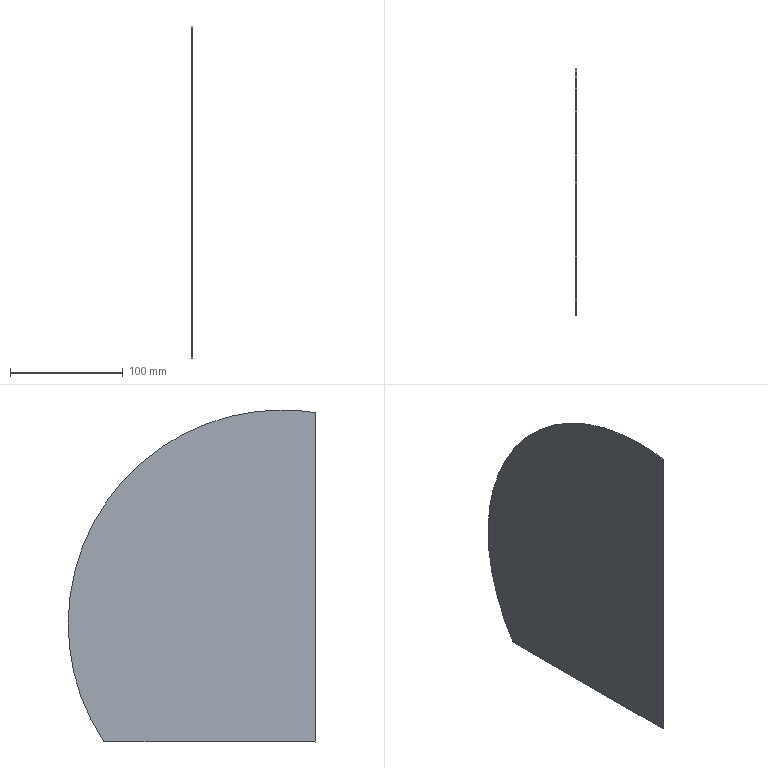Part | STEP file | 09-03 Inner base plate 2 | 1 solid | 6 faces | box 1 x 220 x 295 mm | volume 56061 mm3 | plane 4 | cylinder 2 | commonest cylinder face diameters 380 x2
STEP:
#1=CARTESIAN_POINT('',(0.,0.,0.));
#2=DIRECTION('',(0.,0.,1.));
#3=DIRECTION('',(1.,0.,0.));
#4=AXIS2_PLACEMENT_3D('',#1,#2,#3);
#5=CARTESIAN_POINT('',(1.,30.,295.));
#6=VERTEX_POINT('',#5);
#7=CARTESIAN_POINT('',(1.,0.,292.617));
#8=VERTEX_POINT('',#7);
#9=CARTESIAN_POINT('',(1.,30.,105.));
#10=DIRECTION('',(1.,0.,0.));
#11=DIRECTION('',(0.,0.,1.));
#12=AXIS2_PLACEMENT_3D('',#9,#10,#11);
#13=CIRCLE('',#12,190.);
#14=CARTESIAN_POINT('',(1.,30.,105.));
#15=DIRECTION('',(-1.,0.,0.));
#16=DIRECTION('',(0.,0.,1.));
#17=AXIS2_PLACEMENT_3D('',#14,#15,#16);
#18=CYLINDRICAL_SURFACE('',#17,190.);
#19=CARTESIAN_POINT('',(6.283,0.));
#20=DIRECTION('',(-1.,0.));
#21=VECTOR('',#20,1.);
#22=LINE('',#19,#21);
#23=(GEOMETRIC_REPRESENTATION_CONTEXT(2)PARAMETRIC_REPRESENTATION_CONTEXT()REPRESENTATION_CONTEXT('',''));
#24=DEFINITIONAL_REPRESENTATION('',(#22),#23);
#25=PCURVE('',#18,#24);
#26=CARTESIAN_POINT('',(1.,0.,296.77));
#27=DIRECTION('',(1.,0.,0.));
#28=DIRECTION('',(0.,0.,-1.));
#29=AXIS2_PLACEMENT_3D('',#26,#27,#28);
#30=PLANE('',#29);
#31=CARTESIAN_POINT('',(191.77,30.));
#32=DIRECTION('',(-1.,0.));
#33=AXIS2_PLACEMENT_2D('',#31,#32);
#34=CIRCLE('',#33,190.);
#35=(GEOMETRIC_REPRESENTATION_CONTEXT(2)PARAMETRIC_REPRESENTATION_CONTEXT()REPRESENTATION_CONTEXT('',''));
#36=DEFINITIONAL_REPRESENTATION('',(#34),#35);
#37=PCURVE('',#30,#36);
#38=SURFACE_CURVE('',#13,(#25,#37),.PCURVE_S1.);
#39=EDGE_CURVE('',#6,#8,#38,.T.);
#40=ORIENTED_EDGE('',*,*,#39,.F.);
#41=CARTESIAN_POINT('',(0.,30.,295.));
#42=VERTEX_POINT('',#41);
#43=CARTESIAN_POINT('',(1.,30.,295.));
#44=DIRECTION('',(-1.,0.,0.));
#45=VECTOR('',#44,1.);
#46=LINE('',#43,#45);
#47=CARTESIAN_POINT('',(6.283,0.));
#48=DIRECTION('',(0.,1.));
#49=VECTOR('',#48,1.);
#50=LINE('',#47,#49);
#51=(GEOMETRIC_REPRESENTATION_CONTEXT(2)PARAMETRIC_REPRESENTATION_CONTEXT()REPRESENTATION_CONTEXT('',''));
#52=DEFINITIONAL_REPRESENTATION('',(#50),#51);
#53=PCURVE('',#18,#52);
#54=CARTESIAN_POINT('',(1.,30.,105.));
#55=DIRECTION('',(-1.,0.,0.));
#56=DIRECTION('',(0.,0.,1.));
#57=AXIS2_PLACEMENT_3D('',#54,#55,#56);
#58=CYLINDRICAL_SURFACE('',#57,190.);
#59=CARTESIAN_POINT('',(0.,0.));
#60=DIRECTION('',(0.,1.));
#61=VECTOR('',#60,1.);
#62=LINE('',#59,#61);
#63=(GEOMETRIC_REPRESENTATION_CONTEXT(2)PARAMETRIC_REPRESENTATION_CONTEXT()REPRESENTATION_CONTEXT('',''));
#64=DEFINITIONAL_REPRESENTATION('',(#62),#63);
#65=PCURVE('',#58,#64);
#66=SURFACE_CURVE('',#46,(#53,#65),.PCURVE_S1.);
#67=EDGE_CURVE('',#6,#42,#66,.T.);
#68=ORIENTED_EDGE('',*,*,#67,.T.);
#69=CARTESIAN_POINT('',(0.,0.,292.617));
#70=VERTEX_POINT('',#69);
#71=CARTESIAN_POINT('',(0.,30.,105.));
#72=DIRECTION('',(-1.,0.,0.));
#73=DIRECTION('',(0.,0.,1.));
#74=AXIS2_PLACEMENT_3D('',#71,#72,#73);
#75=CIRCLE('',#74,190.);
#76=CARTESIAN_POINT('',(0.,1.));
#77=DIRECTION('',(1.,0.));
#78=VECTOR('',#77,1.);
#79=LINE('',#76,#78);
#80=(GEOMETRIC_REPRESENTATION_CONTEXT(2)PARAMETRIC_REPRESENTATION_CONTEXT()REPRESENTATION_CONTEXT('',''));
#81=DEFINITIONAL_REPRESENTATION('',(#79),#80);
#82=PCURVE('',#18,#81);
#83=CARTESIAN_POINT('',(0.,0.,296.77));
#84=DIRECTION('',(1.,0.,0.));
#85=DIRECTION('',(0.,0.,-1.));
#86=AXIS2_PLACEMENT_3D('',#83,#84,#85);
#87=PLANE('',#86);
#88=CARTESIAN_POINT('',(1.77,30.));
#89=CARTESIAN_POINT('',(1.77,359.09));
#90=CARTESIAN_POINT('',(286.77,194.545));
#91=CARTESIAN_POINT('',(571.77,30.));
#92=CARTESIAN_POINT('',(286.77,-134.545));
#93=CARTESIAN_POINT('',(1.77,-299.09));
#94=CARTESIAN_POINT('',(1.77,30.));
#95=(BOUNDED_CURVE()B_SPLINE_CURVE(2,(#88,#89,#90,#91,#92,#93,#94),.UNSPECIFIED.,.T.,.F.)B_SPLINE_CURVE_WITH_KNOTS((1,2,2,2,2,1),(-2.094,0.,2.094,4.189,6.283,8.378),.UNSPECIFIED.)CURVE()GEOMETRIC_REPRESENTATION_ITEM()RATIONAL_B_SPLINE_CURVE((1.,0.5,1.,0.5,1.,0.5,1.))REPRESENTATION_ITEM(''));
#96=(GEOMETRIC_REPRESENTATION_CONTEXT(2)PARAMETRIC_REPRESENTATION_CONTEXT()REPRESENTATION_CONTEXT('',''));
#97=DEFINITIONAL_REPRESENTATION('',(#95),#96);
#98=PCURVE('',#87,#97);
#99=SURFACE_CURVE('',#75,(#82,#98),.PCURVE_S1.);
#100=EDGE_CURVE('',#70,#42,#99,.T.);
#101=ORIENTED_EDGE('',*,*,#100,.F.);
#102=CARTESIAN_POINT('',(0.5,0.,292.617));
#103=DIRECTION('',(1.,0.,0.));
#104=VECTOR('',#103,1.);
#105=LINE('',#102,#104);
#106=CARTESIAN_POINT('',(6.125,0.5));
#107=DIRECTION('',(0.,-1.));
#108=VECTOR('',#107,1.);
#109=LINE('',#106,#108);
#110=(GEOMETRIC_REPRESENTATION_CONTEXT(2)PARAMETRIC_REPRESENTATION_CONTEXT()REPRESENTATION_CONTEXT('',''));
#111=DEFINITIONAL_REPRESENTATION('',(#109),#110);
#112=PCURVE('',#18,#111);
#113=CARTESIAN_POINT('',(0.,0.,0.));
#114=DIRECTION('',(0.,1.,0.));
#115=DIRECTION('',(0.,0.,1.));
#116=AXIS2_PLACEMENT_3D('',#113,#114,#115);
#117=PLANE('',#116);
#118=CARTESIAN_POINT('',(292.617,0.5));
#119=DIRECTION('',(0.,1.));
#120=VECTOR('',#119,1.);
#121=LINE('',#118,#120);
#122=(GEOMETRIC_REPRESENTATION_CONTEXT(2)PARAMETRIC_REPRESENTATION_CONTEXT()REPRESENTATION_CONTEXT('',''));
#123=DEFINITIONAL_REPRESENTATION('',(#121),#122);
#124=PCURVE('',#117,#123);
#125=SURFACE_CURVE('',#105,(#112,#124),.PCURVE_S1.);
#126=EDGE_CURVE('',#70,#8,#125,.T.);
#127=ORIENTED_EDGE('',*,*,#126,.T.);
#128=EDGE_LOOP('',(#40,#68,#101,#127));
#129=FACE_BOUND('',#128,.T.);
#130=ADVANCED_FACE('',(#129),#18,.T.);
#131=ORIENTED_EDGE('',*,*,#67,.F.);
#132=CARTESIAN_POINT('',(1.,188.351,0.000000014));
#133=VERTEX_POINT('',#132);
#134=CARTESIAN_POINT('',(1.,30.,105.));
#135=DIRECTION('',(1.,0.,0.));
#136=DIRECTION('',(0.,0.,1.));
#137=AXIS2_PLACEMENT_3D('',#134,#135,#136);
#138=CIRCLE('',#137,190.);
#139=CARTESIAN_POINT('',(6.283,0.));
#140=DIRECTION('',(-1.,0.));
#141=VECTOR('',#140,1.);
#142=LINE('',#139,#141);
#143=(GEOMETRIC_REPRESENTATION_CONTEXT(2)PARAMETRIC_REPRESENTATION_CONTEXT()REPRESENTATION_CONTEXT('',''));
#144=DEFINITIONAL_REPRESENTATION('',(#142),#143);
#145=PCURVE('',#58,#144);
#146=CARTESIAN_POINT('',(191.77,30.));
#147=DIRECTION('',(-1.,0.));
#148=AXIS2_PLACEMENT_2D('',#146,#147);
#149=CIRCLE('',#148,190.);
#150=(GEOMETRIC_REPRESENTATION_CONTEXT(2)PARAMETRIC_REPRESENTATION_CONTEXT()REPRESENTATION_CONTEXT('',''));
#151=DEFINITIONAL_REPRESENTATION('',(#149),#150);
#152=PCURVE('',#30,#151);
#153=SURFACE_CURVE('',#138,(#145,#152),.PCURVE_S1.);
#154=EDGE_CURVE('',#133,#6,#153,.T.);
#155=ORIENTED_EDGE('',*,*,#154,.F.);
#156=CARTESIAN_POINT('',(0.,188.351,0.000000014));
#157=VERTEX_POINT('',#156);
#158=CARTESIAN_POINT('',(0.5,188.351,0.000000027));
#159=DIRECTION('',(1.,0.,0.));
#160=VECTOR('',#159,1.);
#161=LINE('',#158,#160);
#162=CARTESIAN_POINT('',(2.156,0.5));
#163=DIRECTION('',(0.,-1.));
#164=VECTOR('',#163,1.);
#165=LINE('',#162,#164);
#166=(GEOMETRIC_REPRESENTATION_CONTEXT(2)PARAMETRIC_REPRESENTATION_CONTEXT()REPRESENTATION_CONTEXT('',''));
#167=DEFINITIONAL_REPRESENTATION('',(#165),#166);
#168=PCURVE('',#58,#167);
#169=CARTESIAN_POINT('',(0.,188.351,0.));
#170=DIRECTION('',(0.,0.,1.));
#171=DIRECTION('',(0.,-1.,0.));
#172=AXIS2_PLACEMENT_3D('',#169,#170,#171);
#173=PLANE('',#172);
#174=CARTESIAN_POINT('',(-0.000000018,0.5));
#175=DIRECTION('',(0.,1.));
#176=VECTOR('',#175,1.);
#177=LINE('',#174,#176);
#178=(GEOMETRIC_REPRESENTATION_CONTEXT(2)PARAMETRIC_REPRESENTATION_CONTEXT()REPRESENTATION_CONTEXT('',''));
#179=DEFINITIONAL_REPRESENTATION('',(#177),#178);
#180=PCURVE('',#173,#179);
#181=SURFACE_CURVE('',#161,(#168,#180),.PCURVE_S1.);
#182=EDGE_CURVE('',#157,#133,#181,.T.);
#183=ORIENTED_EDGE('',*,*,#182,.F.);
#184=CARTESIAN_POINT('',(0.,30.,105.));
#185=DIRECTION('',(-1.,0.,0.));
#186=DIRECTION('',(0.,0.,1.));
#187=AXIS2_PLACEMENT_3D('',#184,#185,#186);
#188=CIRCLE('',#187,190.);
#189=CARTESIAN_POINT('',(0.,1.));
#190=DIRECTION('',(1.,0.));
#191=VECTOR('',#190,1.);
#192=LINE('',#189,#191);
#193=(GEOMETRIC_REPRESENTATION_CONTEXT(2)PARAMETRIC_REPRESENTATION_CONTEXT()REPRESENTATION_CONTEXT('',''));
#194=DEFINITIONAL_REPRESENTATION('',(#192),#193);
#195=PCURVE('',#58,#194);
#196=CARTESIAN_POINT('',(1.77,30.));
#197=CARTESIAN_POINT('',(1.77,359.09));
#198=CARTESIAN_POINT('',(286.77,194.545));
#199=CARTESIAN_POINT('',(571.77,30.));
#200=CARTESIAN_POINT('',(286.77,-134.545));
#201=CARTESIAN_POINT('',(1.77,-299.09));
#202=CARTESIAN_POINT('',(1.77,30.));
#203=(BOUNDED_CURVE()B_SPLINE_CURVE(2,(#196,#197,#198,#199,#200,#201,#202),.UNSPECIFIED.,.T.,.F.)B_SPLINE_CURVE_WITH_KNOTS((1,2,2,2,2,1),(-2.094,0.,2.094,4.189,6.283,8.378),.UNSPECIFIED.)CURVE()GEOMETRIC_REPRESENTATION_ITEM()RATIONAL_B_SPLINE_CURVE((1.,0.5,1.,0.5,1.,0.5,1.))REPRESENTATION_ITEM(''));
#204=(GEOMETRIC_REPRESENTATION_CONTEXT(2)PARAMETRIC_REPRESENTATION_CONTEXT()REPRESENTATION_CONTEXT('',''));
#205=DEFINITIONAL_REPRESENTATION('',(#203),#204);
#206=PCURVE('',#87,#205);
#207=SURFACE_CURVE('',#188,(#195,#206),.PCURVE_S1.);
#208=EDGE_CURVE('',#42,#157,#207,.T.);
#209=ORIENTED_EDGE('',*,*,#208,.F.);
#210=EDGE_LOOP('',(#131,#155,#183,#209));
#211=FACE_BOUND('',#210,.T.);
#212=ADVANCED_FACE('',(#211),#58,.T.);
#213=ORIENTED_EDGE('',*,*,#154,.T.);
#214=ORIENTED_EDGE('',*,*,#39,.T.);
#215=CARTESIAN_POINT('',(1.,0.,0.));
#216=VERTEX_POINT('',#215);
#217=CARTESIAN_POINT('',(1.,0.,148.385));
#218=DIRECTION('',(0.,0.,-1.));
#219=VECTOR('',#218,1.);
#220=LINE('',#217,#219);
#221=CARTESIAN_POINT('',(148.385,0.));
#222=DIRECTION('',(1.,0.));
#223=VECTOR('',#222,1.);
#224=LINE('',#221,#223);
#225=(GEOMETRIC_REPRESENTATION_CONTEXT(2)PARAMETRIC_REPRESENTATION_CONTEXT()REPRESENTATION_CONTEXT('',''));
#226=DEFINITIONAL_REPRESENTATION('',(#224),#225);
#227=PCURVE('',#30,#226);
#228=CARTESIAN_POINT('',(148.385,1.));
#229=DIRECTION('',(-1.,0.));
#230=VECTOR('',#229,1.);
#231=LINE('',#228,#230);
#232=(GEOMETRIC_REPRESENTATION_CONTEXT(2)PARAMETRIC_REPRESENTATION_CONTEXT()REPRESENTATION_CONTEXT('',''));
#233=DEFINITIONAL_REPRESENTATION('',(#231),#232);
#234=PCURVE('',#117,#233);
#235=SURFACE_CURVE('',#220,(#227,#234),.PCURVE_S1.);
#236=EDGE_CURVE('',#8,#216,#235,.T.);
#237=ORIENTED_EDGE('',*,*,#236,.T.);
#238=CARTESIAN_POINT('',(1.,110.66,0.));
#239=DIRECTION('',(0.,1.,0.));
#240=VECTOR('',#239,1.);
#241=LINE('',#238,#240);
#242=CARTESIAN_POINT('',(296.77,110.66));
#243=DIRECTION('',(0.,1.));
#244=VECTOR('',#243,1.);
#245=LINE('',#242,#244);
#246=(GEOMETRIC_REPRESENTATION_CONTEXT(2)PARAMETRIC_REPRESENTATION_CONTEXT()REPRESENTATION_CONTEXT('',''));
#247=DEFINITIONAL_REPRESENTATION('',(#245),#246);
#248=PCURVE('',#30,#247);
#249=CARTESIAN_POINT('',(77.691,1.));
#250=DIRECTION('',(-1.,0.));
#251=VECTOR('',#250,1.);
#252=LINE('',#249,#251);
#253=(GEOMETRIC_REPRESENTATION_CONTEXT(2)PARAMETRIC_REPRESENTATION_CONTEXT()REPRESENTATION_CONTEXT('',''));
#254=DEFINITIONAL_REPRESENTATION('',(#252),#253);
#255=PCURVE('',#173,#254);
#256=SURFACE_CURVE('',#241,(#248,#255),.PCURVE_S1.);
#257=EDGE_CURVE('',#216,#133,#256,.T.);
#258=ORIENTED_EDGE('',*,*,#257,.T.);
#259=EDGE_LOOP('',(#213,#214,#237,#258));
#260=FACE_BOUND('',#259,.T.);
#261=ADVANCED_FACE('',(#260),#30,.T.);
#262=CARTESIAN_POINT('',(0.,0.,0.));
#263=VERTEX_POINT('',#262);
#264=CARTESIAN_POINT('',(0.,0.,148.385));
#265=DIRECTION('',(0.,0.,-1.));
#266=VECTOR('',#265,1.);
#267=LINE('',#264,#266);
#268=CARTESIAN_POINT('',(148.385,0.));
#269=DIRECTION('',(1.,0.));
#270=VECTOR('',#269,1.);
#271=LINE('',#268,#270);
#272=(GEOMETRIC_REPRESENTATION_CONTEXT(2)PARAMETRIC_REPRESENTATION_CONTEXT()REPRESENTATION_CONTEXT('',''));
#273=DEFINITIONAL_REPRESENTATION('',(#271),#272);
#274=PCURVE('',#87,#273);
#275=CARTESIAN_POINT('',(148.385,0.));
#276=DIRECTION('',(-1.,0.));
#277=VECTOR('',#276,1.);
#278=LINE('',#275,#277);
#279=(GEOMETRIC_REPRESENTATION_CONTEXT(2)PARAMETRIC_REPRESENTATION_CONTEXT()REPRESENTATION_CONTEXT('',''));
#280=DEFINITIONAL_REPRESENTATION('',(#278),#279);
#281=PCURVE('',#117,#280);
#282=SURFACE_CURVE('',#267,(#274,#281),.PCURVE_S1.);
#283=EDGE_CURVE('',#70,#263,#282,.T.);
#284=ORIENTED_EDGE('',*,*,#283,.F.);
#285=ORIENTED_EDGE('',*,*,#100,.T.);
#286=ORIENTED_EDGE('',*,*,#208,.T.);
#287=CARTESIAN_POINT('',(0.,110.66,0.));
#288=DIRECTION('',(0.,1.,0.));
#289=VECTOR('',#288,1.);
#290=LINE('',#287,#289);
#291=CARTESIAN_POINT('',(296.77,110.66));
#292=DIRECTION('',(0.,1.));
#293=VECTOR('',#292,1.);
#294=LINE('',#291,#293);
#295=(GEOMETRIC_REPRESENTATION_CONTEXT(2)PARAMETRIC_REPRESENTATION_CONTEXT()REPRESENTATION_CONTEXT('',''));
#296=DEFINITIONAL_REPRESENTATION('',(#294),#295);
#297=PCURVE('',#87,#296);
#298=CARTESIAN_POINT('',(77.691,0.));
#299=DIRECTION('',(-1.,0.));
#300=VECTOR('',#299,1.);
#301=LINE('',#298,#300);
#302=(GEOMETRIC_REPRESENTATION_CONTEXT(2)PARAMETRIC_REPRESENTATION_CONTEXT()REPRESENTATION_CONTEXT('',''));
#303=DEFINITIONAL_REPRESENTATION('',(#301),#302);
#304=PCURVE('',#173,#303);
#305=SURFACE_CURVE('',#290,(#297,#304),.PCURVE_S1.);
#306=EDGE_CURVE('',#263,#157,#305,.T.);
#307=ORIENTED_EDGE('',*,*,#306,.F.);
#308=EDGE_LOOP('',(#284,#285,#286,#307));
#309=FACE_BOUND('',#308,.T.);
#310=ADVANCED_FACE('',(#309),#87,.F.);
#311=CARTESIAN_POINT('',(0.5,0.,0.));
#312=DIRECTION('',(-1.,0.,0.));
#313=VECTOR('',#312,1.);
#314=LINE('',#311,#313);
#315=CARTESIAN_POINT('',(0.,0.5));
#316=DIRECTION('',(0.,-1.));
#317=VECTOR('',#316,1.);
#318=LINE('',#315,#317);
#319=(GEOMETRIC_REPRESENTATION_CONTEXT(2)PARAMETRIC_REPRESENTATION_CONTEXT()REPRESENTATION_CONTEXT('',''));
#320=DEFINITIONAL_REPRESENTATION('',(#318),#319);
#321=PCURVE('',#117,#320);
#322=CARTESIAN_POINT('',(188.351,0.5));
#323=DIRECTION('',(0.,-1.));
#324=VECTOR('',#323,1.);
#325=LINE('',#322,#324);
#326=(GEOMETRIC_REPRESENTATION_CONTEXT(2)PARAMETRIC_REPRESENTATION_CONTEXT()REPRESENTATION_CONTEXT('',''));
#327=DEFINITIONAL_REPRESENTATION('',(#325),#326);
#328=PCURVE('',#173,#327);
#329=SURFACE_CURVE('',#314,(#321,#328),.PCURVE_S1.);
#330=EDGE_CURVE('',#216,#263,#329,.T.);
#331=ORIENTED_EDGE('',*,*,#330,.F.);
#332=ORIENTED_EDGE('',*,*,#236,.F.);
#333=ORIENTED_EDGE('',*,*,#126,.F.);
#334=ORIENTED_EDGE('',*,*,#283,.T.);
#335=EDGE_LOOP('',(#331,#332,#333,#334));
#336=FACE_BOUND('',#335,.T.);
#337=ADVANCED_FACE('',(#336),#117,.F.);
#338=ORIENTED_EDGE('',*,*,#182,.T.);
#339=ORIENTED_EDGE('',*,*,#257,.F.);
#340=ORIENTED_EDGE('',*,*,#330,.T.);
#341=ORIENTED_EDGE('',*,*,#306,.T.);
#342=EDGE_LOOP('',(#338,#339,#340,#341));
#343=FACE_BOUND('',#342,.T.);
#344=ADVANCED_FACE('',(#343),#173,.F.);
#345=CLOSED_SHELL('',(#130,#212,#261,#310,#337,#344));
#346=MANIFOLD_SOLID_BREP('',#345);
#347=(LENGTH_UNIT()NAMED_UNIT(*)SI_UNIT(.MILLI.,.METRE.));
#348=UNCERTAINTY_MEASURE_WITH_UNIT(LENGTH_MEASURE(0.0000001),#347,'','');
#349=(NAMED_UNIT(*)PLANE_ANGLE_UNIT()SI_UNIT($,.RADIAN.));
#350=(NAMED_UNIT(*)SI_UNIT($,.STERADIAN.)SOLID_ANGLE_UNIT());
#351=(GEOMETRIC_REPRESENTATION_CONTEXT(3)GLOBAL_UNCERTAINTY_ASSIGNED_CONTEXT((#348))GLOBAL_UNIT_ASSIGNED_CONTEXT((#347,#349,#350))REPRESENTATION_CONTEXT('',''));
#352=ADVANCED_BREP_SHAPE_REPRESENTATION('',(#4,#346),#351);